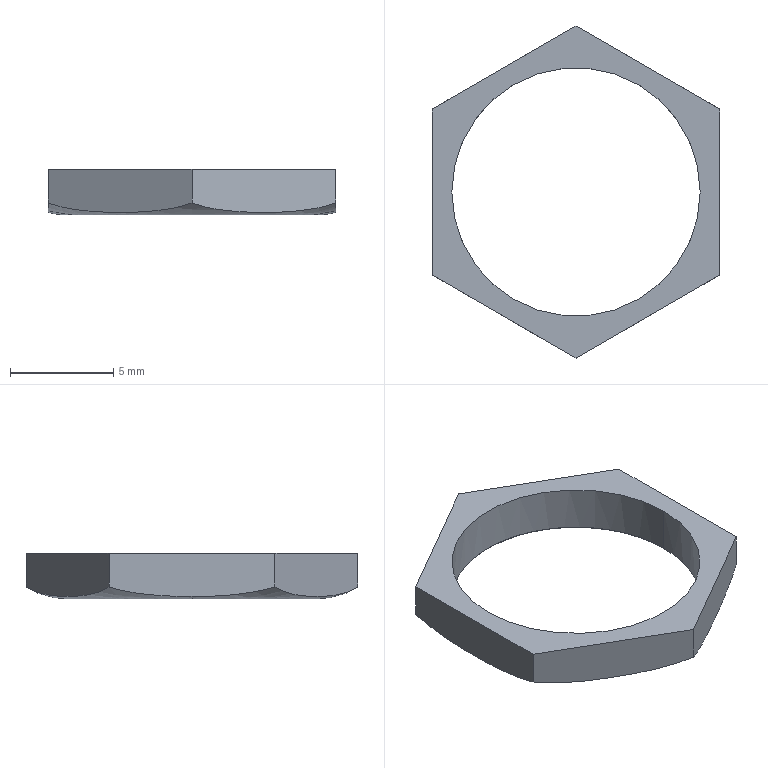Part | SolidWorks | 1 solid | 12 faces | box 13.895 x 16.044 x 2.21 mm | volume 114.581 mm3 | plane 8 | spline 2 | cylinder 2 | commonest cylinder face diameters 12 x2
STEP:
#1=CARTESIAN_POINT('',(6.,-0.00001674,-2.83));
#2=VERTEX_POINT('',#1);
#3=CARTESIAN_POINT('',(-6.,-0.00001674,-2.83));
#4=VERTEX_POINT('',#3);
#5=CARTESIAN_POINT('',(0.,-0.00001674,-2.83));
#6=DIRECTION('',(0.,0.,1.));
#7=DIRECTION('',(1.,0.,0.));
#8=AXIS2_PLACEMENT_3D('',#5,#6,#7);
#9=CIRCLE('',#8,6.);
#10=EDGE_CURVE('',#2,#4,#9,.T.);
#11=ORIENTED_EDGE('',*,*,#10,.T.);
#12=CARTESIAN_POINT('',(0.,-0.00001674,-2.83));
#13=DIRECTION('',(0.,0.,1.));
#14=DIRECTION('',(1.,0.,0.));
#15=AXIS2_PLACEMENT_3D('',#12,#13,#14);
#16=CIRCLE('',#15,6.);
#17=EDGE_CURVE('',#4,#2,#16,.T.);
#18=ORIENTED_EDGE('',*,*,#17,.T.);
#19=EDGE_LOOP('',(#11,#18));
#20=FACE_BOUND('',#19,.T.);
#21=CARTESIAN_POINT('',(-6.017,-0.00001674,-2.83));
#22=VERTEX_POINT('',#21);
#23=CARTESIAN_POINT('',(6.017,-0.00001674,-2.83));
#24=VERTEX_POINT('',#23);
#25=CARTESIAN_POINT('',(-6.017,-0.00001674,-2.83));
#26=CARTESIAN_POINT('',(-6.017,-12.033,-2.83));
#27=CARTESIAN_POINT('',(6.017,-12.033,-2.83));
#28=CARTESIAN_POINT('',(6.017,-0.00001674,-2.83));
#29=(BOUNDED_CURVE()B_SPLINE_CURVE(3,(#25,#26,#27,#28),.UNSPECIFIED.,.F.,.T.)B_SPLINE_CURVE_WITH_KNOTS((4,4),(0.,1.),.UNSPECIFIED.)CURVE()GEOMETRIC_REPRESENTATION_ITEM()RATIONAL_B_SPLINE_CURVE((1.,0.3333,0.3333,1.))REPRESENTATION_ITEM(''));
#30=EDGE_CURVE('',#22,#24,#29,.T.);
#31=ORIENTED_EDGE('',*,*,#30,.F.);
#32=CARTESIAN_POINT('',(6.017,-0.00001674,-2.83));
#33=CARTESIAN_POINT('',(6.017,12.033,-2.83));
#34=CARTESIAN_POINT('',(-6.017,12.033,-2.83));
#35=CARTESIAN_POINT('',(-6.017,-0.00001674,-2.83));
#36=(BOUNDED_CURVE()B_SPLINE_CURVE(3,(#32,#33,#34,#35),.UNSPECIFIED.,.F.,.T.)B_SPLINE_CURVE_WITH_KNOTS((4,4),(0.,1.),.UNSPECIFIED.)CURVE()GEOMETRIC_REPRESENTATION_ITEM()RATIONAL_B_SPLINE_CURVE((1.,0.3333,0.3333,1.))REPRESENTATION_ITEM(''));
#37=EDGE_CURVE('',#24,#22,#36,.T.);
#38=ORIENTED_EDGE('',*,*,#37,.F.);
#39=EDGE_LOOP('',(#31,#38));
#40=FACE_OUTER_BOUND('',#39,.T.);
#41=CARTESIAN_POINT('',(0.,6.016,-2.83));
#42=DIRECTION('',(0.,0.,1.));
#43=DIRECTION('',(1.,0.,0.));
#44=AXIS2_PLACEMENT_3D('',#41,#42,#43);
#45=PLANE('',#44);
#46=ADVANCED_FACE('',(#20,#40),#45,.F.);
#47=CARTESIAN_POINT('',(-6.947,-0.00001674,-2.715));
#48=VERTEX_POINT('',#47);
#49=CARTESIAN_POINT('',(-6.017,-0.00001674,0.9919));
#50=DIRECTION('',(0.,-1.,0.));
#51=DIRECTION('',(-1.,0.,0.));
#52=AXIS2_PLACEMENT_3D('',#49,#50,#51);
#53=CIRCLE('',#52,3.822);
#54=EDGE_CURVE('',#48,#22,#53,.T.);
#55=ORIENTED_EDGE('',*,*,#54,.F.);
#56=CARTESIAN_POINT('',(-6.947,4.011,-2.262));
#57=VERTEX_POINT('',#56);
#58=CARTESIAN_POINT('',(-6.947,4.011,-2.262));
#59=CARTESIAN_POINT('',(-6.947,3.728,-2.349));
#60=CARTESIAN_POINT('',(-6.947,3.267,-2.46));
#61=CARTESIAN_POINT('',(-6.947,2.666,-2.557));
#62=CARTESIAN_POINT('',(-6.947,2.349,-2.597));
#63=CARTESIAN_POINT('',(-6.947,2.187,-2.614));
#64=CARTESIAN_POINT('',(-6.947,2.104,-2.623));
#65=CARTESIAN_POINT('',(-6.947,2.063,-2.627));
#66=CARTESIAN_POINT('',(-6.947,2.045,-2.628));
#67=CARTESIAN_POINT('',(-6.947,2.033,-2.63));
#68=CARTESIAN_POINT('',(-6.947,2.026,-2.63));
#69=CARTESIAN_POINT('',(-6.947,1.422,-2.687));
#70=CARTESIAN_POINT('',(-6.947,0.7486,-2.715));
#71=CARTESIAN_POINT('',(-6.947,-0.00001674,-2.715));
#72=B_SPLINE_CURVE_WITH_KNOTS('',3,(#58,#59,#60,#61,#62,#63,#64,#65,#66,#67,#68,#69,#70,#71),.UNSPECIFIED.,.F.,.F.,(4,1,1,1,1,1,1,2,2,4),(0.,0.25,0.375,0.4375,0.4688,0.4844,0.4922,0.4961,0.5,1.),.UNSPECIFIED.);
#73=EDGE_CURVE('',#57,#48,#72,.T.);
#74=ORIENTED_EDGE('',*,*,#73,.F.);
#75=CARTESIAN_POINT('',(0.,8.022,-2.262));
#76=VERTEX_POINT('',#75);
#77=CARTESIAN_POINT('',(0.,8.022,-2.262));
#78=CARTESIAN_POINT('',(-0.245,7.881,-2.349));
#79=CARTESIAN_POINT('',(-0.6442,7.65,-2.461));
#80=CARTESIAN_POINT('',(-1.165,7.349,-2.557));
#81=CARTESIAN_POINT('',(-1.439,7.191,-2.597));
#82=CARTESIAN_POINT('',(-1.58,7.11,-2.614));
#83=CARTESIAN_POINT('',(-1.651,7.069,-2.623));
#84=CARTESIAN_POINT('',(-1.687,7.048,-2.627));
#85=CARTESIAN_POINT('',(-1.702,7.039,-2.628));
#86=CARTESIAN_POINT('',(-1.713,7.033,-2.63));
#87=CARTESIAN_POINT('',(-1.719,7.03,-2.63));
#88=CARTESIAN_POINT('',(-2.242,6.728,-2.687));
#89=CARTESIAN_POINT('',(-2.826,6.391,-2.715));
#90=CARTESIAN_POINT('',(-3.797,5.83,-2.715));
#91=CARTESIAN_POINT('',(-4.259,5.563,-2.705));
#92=CARTESIAN_POINT('',(-4.756,5.276,-2.674));
#93=CARTESIAN_POINT('',(-4.994,5.139,-2.654));
#94=CARTESIAN_POINT('',(-5.11,5.072,-2.643));
#95=CARTESIAN_POINT('',(-5.167,5.039,-2.637));
#96=CARTESIAN_POINT('',(-5.196,5.022,-2.634));
#97=CARTESIAN_POINT('',(-5.208,5.015,-2.632));
#98=CARTESIAN_POINT('',(-5.216,5.01,-2.632));
#99=CARTESIAN_POINT('',(-5.219,5.009,-2.631));
#100=CARTESIAN_POINT('',(-5.883,4.626,-2.559));
#101=CARTESIAN_POINT('',(-6.457,4.294,-2.436));
#102=CARTESIAN_POINT('',(-6.947,4.011,-2.262));
#103=B_SPLINE_CURVE_WITH_KNOTS('',3,(#77,#78,#79,#80,#81,#82,#83,#84,#85,#86,#87,#88,#89,#90,#91,#92,#93,#94,#95,#96,#97,#98,#99,#100,#101,#102),.UNSPECIFIED.,.F.,.F.,(4,1,1,1,1,1,1,2,2,2,1,1,1,1,1,1,2,2,4),(0.,0.125,0.1875,0.2187,0.2344,0.2422,0.2461,0.248,0.25,0.5,0.625,0.6875,0.7187,0.7344,0.7422,0.7461,0.748,0.75,1.),.UNSPECIFIED.);
#104=EDGE_CURVE('',#76,#57,#103,.T.);
#105=ORIENTED_EDGE('',*,*,#104,.F.);
#106=CARTESIAN_POINT('',(6.947,4.011,-2.262));
#107=VERTEX_POINT('',#106);
#108=CARTESIAN_POINT('',(6.947,4.011,-2.262));
#109=CARTESIAN_POINT('',(6.702,4.152,-2.349));
#110=CARTESIAN_POINT('',(6.303,4.383,-2.461));
#111=CARTESIAN_POINT('',(5.782,4.684,-2.557));
#112=CARTESIAN_POINT('',(5.508,4.842,-2.597));
#113=CARTESIAN_POINT('',(5.367,4.923,-2.614));
#114=CARTESIAN_POINT('',(5.296,4.964,-2.623));
#115=CARTESIAN_POINT('',(5.26,4.985,-2.627));
#116=CARTESIAN_POINT('',(5.245,4.994,-2.628));
#117=CARTESIAN_POINT('',(5.235,5.,-2.63));
#118=CARTESIAN_POINT('',(5.228,5.003,-2.63));
#119=CARTESIAN_POINT('',(4.706,5.305,-2.687));
#120=CARTESIAN_POINT('',(4.122,5.642,-2.715));
#121=CARTESIAN_POINT('',(3.15,6.203,-2.715));
#122=CARTESIAN_POINT('',(2.688,6.47,-2.705));
#123=CARTESIAN_POINT('',(2.191,6.757,-2.674));
#124=CARTESIAN_POINT('',(1.954,6.894,-2.654));
#125=CARTESIAN_POINT('',(1.837,6.961,-2.643));
#126=CARTESIAN_POINT('',(1.78,6.994,-2.637));
#127=CARTESIAN_POINT('',(1.751,7.011,-2.634));
#128=CARTESIAN_POINT('',(1.739,7.018,-2.632));
#129=CARTESIAN_POINT('',(1.731,7.023,-2.632));
#130=CARTESIAN_POINT('',(1.728,7.024,-2.631));
#131=CARTESIAN_POINT('',(1.065,7.407,-2.559));
#132=CARTESIAN_POINT('',(0.4902,7.739,-2.436));
#133=CARTESIAN_POINT('',(0.,8.022,-2.262));
#134=B_SPLINE_CURVE_WITH_KNOTS('',3,(#108,#109,#110,#111,#112,#113,#114,#115,#116,#117,#118,#119,#120,#121,#122,#123,#124,#125,#126,#127,#128,#129,#130,#131,#132,#133),.UNSPECIFIED.,.F.,.F.,(4,1,1,1,1,1,1,2,2,2,1,1,1,1,1,1,2,2,4),(0.,0.125,0.1875,0.2188,0.2344,0.2422,0.2461,0.248,0.25,0.5,0.625,0.6875,0.7187,0.7344,0.7422,0.7461,0.748,0.75,1.),.UNSPECIFIED.);
#135=EDGE_CURVE('',#107,#76,#134,.T.);
#136=ORIENTED_EDGE('',*,*,#135,.F.);
#137=CARTESIAN_POINT('',(6.947,-0.00001674,-2.715));
#138=VERTEX_POINT('',#137);
#139=CARTESIAN_POINT('',(6.947,-0.00001674,-2.715));
#140=CARTESIAN_POINT('',(6.947,0.3741,-2.715));
#141=CARTESIAN_POINT('',(6.947,0.9074,-2.705));
#142=CARTESIAN_POINT('',(6.947,1.481,-2.674));
#143=CARTESIAN_POINT('',(6.947,1.755,-2.654));
#144=CARTESIAN_POINT('',(6.947,1.889,-2.643));
#145=CARTESIAN_POINT('',(6.947,1.956,-2.637));
#146=CARTESIAN_POINT('',(6.947,1.989,-2.634));
#147=CARTESIAN_POINT('',(6.947,2.003,-2.632));
#148=CARTESIAN_POINT('',(6.947,2.012,-2.632));
#149=CARTESIAN_POINT('',(6.947,2.016,-2.631));
#150=CARTESIAN_POINT('',(6.947,2.782,-2.559));
#151=CARTESIAN_POINT('',(6.947,3.445,-2.436));
#152=CARTESIAN_POINT('',(6.947,4.011,-2.262));
#153=B_SPLINE_CURVE_WITH_KNOTS('',3,(#139,#140,#141,#142,#143,#144,#145,#146,#147,#148,#149,#150,#151,#152),.UNSPECIFIED.,.F.,.F.,(4,1,1,1,1,1,1,2,2,4),(0.,0.25,0.375,0.4375,0.4688,0.4844,0.4922,0.4961,0.5,1.),.UNSPECIFIED.);
#154=EDGE_CURVE('',#138,#107,#153,.T.);
#155=ORIENTED_EDGE('',*,*,#154,.F.);
#156=CARTESIAN_POINT('',(6.017,-0.00001674,0.9919));
#157=DIRECTION('',(0.,1.,0.));
#158=DIRECTION('',(1.,0.,0.));
#159=AXIS2_PLACEMENT_3D('',#156,#157,#158);
#160=CIRCLE('',#159,3.822);
#161=EDGE_CURVE('',#138,#24,#160,.T.);
#162=ORIENTED_EDGE('',*,*,#161,.T.);
#163=ORIENTED_EDGE('',*,*,#37,.T.);
#164=EDGE_LOOP('',(#55,#74,#105,#136,#155,#162,#163));
#165=FACE_OUTER_BOUND('',#164,.T.);
#166=CARTESIAN_POINT('',(8.033,-0.00001674,-2.255));
#167=CARTESIAN_POINT('',(8.033,16.066,-2.255));
#168=CARTESIAN_POINT('',(-8.033,16.066,-2.255));
#169=CARTESIAN_POINT('',(-8.033,-0.00001674,-2.255));
#170=CARTESIAN_POINT('',(7.423,-0.00001674,-2.633));
#171=CARTESIAN_POINT('',(7.423,14.847,-2.633));
#172=CARTESIAN_POINT('',(-7.423,14.847,-2.633));
#173=CARTESIAN_POINT('',(-7.423,-0.00001674,-2.633));
#174=CARTESIAN_POINT('',(6.734,-0.00001674,-2.83));
#175=CARTESIAN_POINT('',(6.734,13.467,-2.83));
#176=CARTESIAN_POINT('',(-6.734,13.467,-2.83));
#177=CARTESIAN_POINT('',(-6.734,-0.00001674,-2.83));
#178=CARTESIAN_POINT('',(6.017,-0.00001674,-2.83));
#179=CARTESIAN_POINT('',(6.017,12.033,-2.83));
#180=CARTESIAN_POINT('',(-6.017,12.033,-2.83));
#181=CARTESIAN_POINT('',(-6.017,-0.00001674,-2.83));
#182=(BOUNDED_SURFACE()B_SPLINE_SURFACE(3,3,((#166,#167,#168,#169),(#170,#171,#172,#173),(#174,#175,#176,#177),(#178,#179,#180,#181)),.UNSPECIFIED.,.F.,.F.,.F.)B_SPLINE_SURFACE_WITH_KNOTS((4,4),(4,4),(0.,1.),(0.,1.),.UNSPECIFIED.)GEOMETRIC_REPRESENTATION_ITEM()RATIONAL_B_SPLINE_SURFACE(((1.,0.3333,0.3333,1.),(0.9744,0.3248,0.3248,0.9744),(0.9744,0.3248,0.3248,0.9744),(1.,0.3333,0.3333,1.)))REPRESENTATION_ITEM('')SURFACE());
#183=ADVANCED_FACE('',(#165),#182,.T.);
#184=CARTESIAN_POINT('',(-6.,-0.00001674,-0.6197));
#185=VERTEX_POINT('',#184);
#186=CARTESIAN_POINT('',(-6.,-0.00001674,-0.6197));
#187=DIRECTION('',(0.,0.,1.));
#188=VECTOR('',#187,1000.);
#189=LINE('',#186,#188);
#190=EDGE_CURVE('',#4,#185,#189,.T.);
#191=ORIENTED_EDGE('',*,*,#190,.F.);
#192=ORIENTED_EDGE('',*,*,#10,.F.);
#193=CARTESIAN_POINT('',(6.,-0.00001674,-0.6197));
#194=VERTEX_POINT('',#193);
#195=CARTESIAN_POINT('',(6.,-0.00001674,-0.6197));
#196=DIRECTION('',(0.,0.,1.));
#197=VECTOR('',#196,1000.);
#198=LINE('',#195,#197);
#199=EDGE_CURVE('',#2,#194,#198,.T.);
#200=ORIENTED_EDGE('',*,*,#199,.T.);
#201=CARTESIAN_POINT('',(0.,-0.00001674,-0.6197));
#202=DIRECTION('',(0.,0.,1.));
#203=DIRECTION('',(1.,0.,0.));
#204=AXIS2_PLACEMENT_3D('',#201,#202,#203);
#205=CIRCLE('',#204,6.);
#206=EDGE_CURVE('',#194,#185,#205,.T.);
#207=ORIENTED_EDGE('',*,*,#206,.T.);
#208=EDGE_LOOP('',(#191,#192,#200,#207));
#209=FACE_OUTER_BOUND('',#208,.T.);
#210=CARTESIAN_POINT('',(0.,-0.00001674,-0.6197));
#211=DIRECTION('',(0.,0.,1.));
#212=DIRECTION('',(1.,0.,0.));
#213=AXIS2_PLACEMENT_3D('',#210,#211,#212);
#214=CYLINDRICAL_SURFACE('',#213,6.);
#215=ADVANCED_FACE('',(#209),#214,.F.);
#216=CARTESIAN_POINT('',(6.947,4.011,-0.6197));
#217=VERTEX_POINT('',#216);
#218=CARTESIAN_POINT('',(6.947,-4.011,-0.6197));
#219=VERTEX_POINT('',#218);
#220=CARTESIAN_POINT('',(6.947,6.,-0.6197));
#221=DIRECTION('',(0.,-1.,0.));
#222=VECTOR('',#221,1000.);
#223=LINE('',#220,#222);
#224=EDGE_CURVE('',#217,#219,#223,.T.);
#225=ORIENTED_EDGE('',*,*,#224,.T.);
#226=CARTESIAN_POINT('',(6.947,-4.011,-2.262));
#227=VERTEX_POINT('',#226);
#228=CARTESIAN_POINT('',(6.947,-4.011,-2.83));
#229=DIRECTION('',(0.,0.,1.));
#230=VECTOR('',#229,1000.);
#231=LINE('',#228,#230);
#232=EDGE_CURVE('',#227,#219,#231,.T.);
#233=ORIENTED_EDGE('',*,*,#232,.F.);
#234=CARTESIAN_POINT('',(6.947,-4.011,-2.262));
#235=CARTESIAN_POINT('',(6.947,-3.728,-2.349));
#236=CARTESIAN_POINT('',(6.947,-3.267,-2.46));
#237=CARTESIAN_POINT('',(6.947,-2.666,-2.557));
#238=CARTESIAN_POINT('',(6.947,-2.349,-2.597));
#239=CARTESIAN_POINT('',(6.947,-2.187,-2.614));
#240=CARTESIAN_POINT('',(6.947,-2.104,-2.623));
#241=CARTESIAN_POINT('',(6.947,-2.063,-2.627));
#242=CARTESIAN_POINT('',(6.947,-2.045,-2.628));
#243=CARTESIAN_POINT('',(6.947,-2.033,-2.63));
#244=CARTESIAN_POINT('',(6.947,-2.026,-2.63));
#245=CARTESIAN_POINT('',(6.947,-1.423,-2.687));
#246=CARTESIAN_POINT('',(6.947,-0.7487,-2.715));
#247=CARTESIAN_POINT('',(6.947,-0.00001674,-2.715));
#248=B_SPLINE_CURVE_WITH_KNOTS('',3,(#234,#235,#236,#237,#238,#239,#240,#241,#242,#243,#244,#245,#246,#247),.UNSPECIFIED.,.F.,.F.,(4,1,1,1,1,1,1,2,2,4),(0.,0.25,0.375,0.4375,0.4687,0.4844,0.4922,0.4961,0.5,1.),.UNSPECIFIED.);
#249=EDGE_CURVE('',#227,#138,#248,.T.);
#250=ORIENTED_EDGE('',*,*,#249,.T.);
#251=ORIENTED_EDGE('',*,*,#154,.T.);
#252=CARTESIAN_POINT('',(6.947,4.011,-2.83));
#253=DIRECTION('',(0.,0.,-1.));
#254=VECTOR('',#253,1000.);
#255=LINE('',#252,#254);
#256=EDGE_CURVE('',#217,#107,#255,.T.);
#257=ORIENTED_EDGE('',*,*,#256,.F.);
#258=EDGE_LOOP('',(#225,#233,#250,#251,#257));
#259=FACE_OUTER_BOUND('',#258,.T.);
#260=CARTESIAN_POINT('',(6.947,-4.011,-2.83));
#261=DIRECTION('',(1.,0.,0.));
#262=DIRECTION('',(0.,1.,0.));
#263=AXIS2_PLACEMENT_3D('',#260,#261,#262);
#264=PLANE('',#263);
#265=ADVANCED_FACE('',(#259),#264,.T.);
#266=CARTESIAN_POINT('',(0.,-8.022,-0.6197));
#267=VERTEX_POINT('',#266);
#268=CARTESIAN_POINT('',(6.947,-4.011,-0.6197));
#269=DIRECTION('',(-0.866,-0.5,0.));
#270=VECTOR('',#269,1000.);
#271=LINE('',#268,#270);
#272=EDGE_CURVE('',#219,#267,#271,.T.);
#273=ORIENTED_EDGE('',*,*,#272,.T.);
#274=CARTESIAN_POINT('',(0.,-8.022,-2.262));
#275=VERTEX_POINT('',#274);
#276=CARTESIAN_POINT('',(0.,-8.022,-2.83));
#277=DIRECTION('',(0.,0.,1.));
#278=VECTOR('',#277,1000.);
#279=LINE('',#276,#278);
#280=EDGE_CURVE('',#275,#267,#279,.T.);
#281=ORIENTED_EDGE('',*,*,#280,.F.);
#282=CARTESIAN_POINT('',(0.,-8.022,-2.262));
#283=CARTESIAN_POINT('',(0.245,-7.881,-2.349));
#284=CARTESIAN_POINT('',(0.6442,-7.65,-2.461));
#285=CARTESIAN_POINT('',(1.165,-7.349,-2.557));
#286=CARTESIAN_POINT('',(1.439,-7.191,-2.597));
#287=CARTESIAN_POINT('',(1.58,-7.11,-2.614));
#288=CARTESIAN_POINT('',(1.651,-7.069,-2.623));
#289=CARTESIAN_POINT('',(1.687,-7.048,-2.627));
#290=CARTESIAN_POINT('',(1.702,-7.039,-2.628));
#291=CARTESIAN_POINT('',(1.713,-7.033,-2.63));
#292=CARTESIAN_POINT('',(1.719,-7.03,-2.63));
#293=CARTESIAN_POINT('',(2.242,-6.728,-2.687));
#294=CARTESIAN_POINT('',(2.826,-6.391,-2.715));
#295=CARTESIAN_POINT('',(3.797,-5.83,-2.715));
#296=CARTESIAN_POINT('',(4.259,-5.563,-2.705));
#297=CARTESIAN_POINT('',(4.756,-5.276,-2.674));
#298=CARTESIAN_POINT('',(4.994,-5.139,-2.654));
#299=CARTESIAN_POINT('',(5.11,-5.072,-2.643));
#300=CARTESIAN_POINT('',(5.167,-5.039,-2.637));
#301=CARTESIAN_POINT('',(5.196,-5.022,-2.634));
#302=CARTESIAN_POINT('',(5.208,-5.015,-2.632));
#303=CARTESIAN_POINT('',(5.216,-5.01,-2.632));
#304=CARTESIAN_POINT('',(5.219,-5.009,-2.631));
#305=CARTESIAN_POINT('',(5.883,-4.626,-2.559));
#306=CARTESIAN_POINT('',(6.457,-4.294,-2.436));
#307=CARTESIAN_POINT('',(6.947,-4.011,-2.262));
#308=B_SPLINE_CURVE_WITH_KNOTS('',3,(#282,#283,#284,#285,#286,#287,#288,#289,#290,#291,#292,#293,#294,#295,#296,#297,#298,#299,#300,#301,#302,#303,#304,#305,#306,#307),.UNSPECIFIED.,.F.,.F.,(4,1,1,1,1,1,1,2,2,2,1,1,1,1,1,1,2,2,4),(0.,0.125,0.1875,0.2188,0.2344,0.2422,0.2461,0.248,0.25,0.5,0.625,0.6875,0.7187,0.7344,0.7422,0.7461,0.748,0.75,1.),.UNSPECIFIED.);
#309=EDGE_CURVE('',#275,#227,#308,.T.);
#310=ORIENTED_EDGE('',*,*,#309,.T.);
#311=ORIENTED_EDGE('',*,*,#232,.T.);
#312=EDGE_LOOP('',(#273,#281,#310,#311));
#313=FACE_OUTER_BOUND('',#312,.T.);
#314=CARTESIAN_POINT('',(0.,-8.022,-2.83));
#315=DIRECTION('',(0.5,-0.866,0.));
#316=DIRECTION('',(0.,0.,-1.));
#317=AXIS2_PLACEMENT_3D('',#314,#315,#316);
#318=PLANE('',#317);
#319=ADVANCED_FACE('',(#313),#318,.T.);
#320=CARTESIAN_POINT('',(-6.947,-4.011,-0.6197));
#321=VERTEX_POINT('',#320);
#322=CARTESIAN_POINT('',(0.,-8.022,-0.6197));
#323=DIRECTION('',(-0.866,0.5,0.));
#324=VECTOR('',#323,1000.);
#325=LINE('',#322,#324);
#326=EDGE_CURVE('',#267,#321,#325,.T.);
#327=ORIENTED_EDGE('',*,*,#326,.T.);
#328=CARTESIAN_POINT('',(-6.947,-4.011,-2.262));
#329=VERTEX_POINT('',#328);
#330=CARTESIAN_POINT('',(-6.947,-4.011,-2.83));
#331=DIRECTION('',(0.,0.,1.));
#332=VECTOR('',#331,1000.);
#333=LINE('',#330,#332);
#334=EDGE_CURVE('',#329,#321,#333,.T.);
#335=ORIENTED_EDGE('',*,*,#334,.F.);
#336=CARTESIAN_POINT('',(-6.947,-4.011,-2.262));
#337=CARTESIAN_POINT('',(-6.702,-4.152,-2.349));
#338=CARTESIAN_POINT('',(-6.303,-4.383,-2.461));
#339=CARTESIAN_POINT('',(-5.782,-4.684,-2.557));
#340=CARTESIAN_POINT('',(-5.508,-4.842,-2.597));
#341=CARTESIAN_POINT('',(-5.367,-4.923,-2.614));
#342=CARTESIAN_POINT('',(-5.296,-4.964,-2.623));
#343=CARTESIAN_POINT('',(-5.26,-4.985,-2.627));
#344=CARTESIAN_POINT('',(-5.245,-4.994,-2.628));
#345=CARTESIAN_POINT('',(-5.235,-5.,-2.63));
#346=CARTESIAN_POINT('',(-5.228,-5.003,-2.63));
#347=CARTESIAN_POINT('',(-4.706,-5.305,-2.687));
#348=CARTESIAN_POINT('',(-4.122,-5.642,-2.715));
#349=CARTESIAN_POINT('',(-3.15,-6.204,-2.715));
#350=CARTESIAN_POINT('',(-2.688,-6.47,-2.705));
#351=CARTESIAN_POINT('',(-2.191,-6.757,-2.674));
#352=CARTESIAN_POINT('',(-1.954,-6.894,-2.654));
#353=CARTESIAN_POINT('',(-1.837,-6.961,-2.643));
#354=CARTESIAN_POINT('',(-1.78,-6.994,-2.637));
#355=CARTESIAN_POINT('',(-1.751,-7.011,-2.634));
#356=CARTESIAN_POINT('',(-1.739,-7.018,-2.632));
#357=CARTESIAN_POINT('',(-1.731,-7.023,-2.632));
#358=CARTESIAN_POINT('',(-1.728,-7.024,-2.631));
#359=CARTESIAN_POINT('',(-1.065,-7.407,-2.559));
#360=CARTESIAN_POINT('',(-0.4902,-7.739,-2.436));
#361=CARTESIAN_POINT('',(0.,-8.022,-2.262));
#362=B_SPLINE_CURVE_WITH_KNOTS('',3,(#336,#337,#338,#339,#340,#341,#342,#343,#344,#345,#346,#347,#348,#349,#350,#351,#352,#353,#354,#355,#356,#357,#358,#359,#360,#361),.UNSPECIFIED.,.F.,.F.,(4,1,1,1,1,1,1,2,2,2,1,1,1,1,1,1,2,2,4),(0.,0.125,0.1875,0.2187,0.2344,0.2422,0.2461,0.248,0.25,0.5,0.625,0.6875,0.7188,0.7344,0.7422,0.7461,0.748,0.75,1.),.UNSPECIFIED.);
#363=EDGE_CURVE('',#329,#275,#362,.T.);
#364=ORIENTED_EDGE('',*,*,#363,.T.);
#365=ORIENTED_EDGE('',*,*,#280,.T.);
#366=EDGE_LOOP('',(#327,#335,#364,#365));
#367=FACE_OUTER_BOUND('',#366,.T.);
#368=CARTESIAN_POINT('',(-6.947,-4.011,-2.83));
#369=DIRECTION('',(-0.5,-0.866,0.));
#370=DIRECTION('',(-0.866,0.5,0.));
#371=AXIS2_PLACEMENT_3D('',#368,#369,#370);
#372=PLANE('',#371);
#373=ADVANCED_FACE('',(#367),#372,.T.);
#374=CARTESIAN_POINT('',(-6.947,4.011,-0.6197));
#375=VERTEX_POINT('',#374);
#376=CARTESIAN_POINT('',(-6.947,6.,-0.6197));
#377=DIRECTION('',(0.,1.,0.));
#378=VECTOR('',#377,1000.);
#379=LINE('',#376,#378);
#380=EDGE_CURVE('',#321,#375,#379,.T.);
#381=ORIENTED_EDGE('',*,*,#380,.T.);
#382=CARTESIAN_POINT('',(-6.947,4.011,-2.83));
#383=DIRECTION('',(0.,0.,1.));
#384=VECTOR('',#383,1000.);
#385=LINE('',#382,#384);
#386=EDGE_CURVE('',#57,#375,#385,.T.);
#387=ORIENTED_EDGE('',*,*,#386,.F.);
#388=ORIENTED_EDGE('',*,*,#73,.T.);
#389=CARTESIAN_POINT('',(-6.947,-0.00001674,-2.715));
#390=CARTESIAN_POINT('',(-6.947,-0.3741,-2.715));
#391=CARTESIAN_POINT('',(-6.947,-0.9074,-2.705));
#392=CARTESIAN_POINT('',(-6.947,-1.481,-2.674));
#393=CARTESIAN_POINT('',(-6.947,-1.755,-2.654));
#394=CARTESIAN_POINT('',(-6.947,-1.889,-2.643));
#395=CARTESIAN_POINT('',(-6.947,-1.956,-2.637));
#396=CARTESIAN_POINT('',(-6.947,-1.989,-2.634));
#397=CARTESIAN_POINT('',(-6.947,-2.003,-2.632));
#398=CARTESIAN_POINT('',(-6.947,-2.012,-2.632));
#399=CARTESIAN_POINT('',(-6.947,-2.016,-2.631));
#400=CARTESIAN_POINT('',(-6.947,-2.782,-2.559));
#401=CARTESIAN_POINT('',(-6.947,-3.445,-2.436));
#402=CARTESIAN_POINT('',(-6.947,-4.011,-2.262));
#403=B_SPLINE_CURVE_WITH_KNOTS('',3,(#389,#390,#391,#392,#393,#394,#395,#396,#397,#398,#399,#400,#401,#402),.UNSPECIFIED.,.F.,.F.,(4,1,1,1,1,1,1,2,2,4),(0.,0.25,0.375,0.4375,0.4687,0.4844,0.4922,0.4961,0.5,1.),.UNSPECIFIED.);
#404=EDGE_CURVE('',#48,#329,#403,.T.);
#405=ORIENTED_EDGE('',*,*,#404,.T.);
#406=ORIENTED_EDGE('',*,*,#334,.T.);
#407=EDGE_LOOP('',(#381,#387,#388,#405,#406));
#408=FACE_OUTER_BOUND('',#407,.T.);
#409=CARTESIAN_POINT('',(-6.947,4.011,-2.83));
#410=DIRECTION('',(-1.,0.,0.));
#411=DIRECTION('',(0.,1.,0.));
#412=AXIS2_PLACEMENT_3D('',#409,#410,#411);
#413=PLANE('',#412);
#414=ADVANCED_FACE('',(#408),#413,.T.);
#415=CARTESIAN_POINT('',(0.,8.022,-0.6197));
#416=VERTEX_POINT('',#415);
#417=CARTESIAN_POINT('',(-6.947,4.011,-0.6197));
#418=DIRECTION('',(0.866,0.5,0.));
#419=VECTOR('',#418,1000.);
#420=LINE('',#417,#419);
#421=EDGE_CURVE('',#375,#416,#420,.T.);
#422=ORIENTED_EDGE('',*,*,#421,.T.);
#423=CARTESIAN_POINT('',(0.,8.022,-2.83));
#424=DIRECTION('',(0.,0.,1.));
#425=VECTOR('',#424,1000.);
#426=LINE('',#423,#425);
#427=EDGE_CURVE('',#76,#416,#426,.T.);
#428=ORIENTED_EDGE('',*,*,#427,.F.);
#429=ORIENTED_EDGE('',*,*,#104,.T.);
#430=ORIENTED_EDGE('',*,*,#386,.T.);
#431=EDGE_LOOP('',(#422,#428,#429,#430));
#432=FACE_OUTER_BOUND('',#431,.T.);
#433=CARTESIAN_POINT('',(0.,8.022,-2.83));
#434=DIRECTION('',(-0.5,0.866,0.));
#435=DIRECTION('',(0.,0.,1.));
#436=AXIS2_PLACEMENT_3D('',#433,#434,#435);
#437=PLANE('',#436);
#438=ADVANCED_FACE('',(#432),#437,.T.);
#439=CARTESIAN_POINT('',(0.,8.022,-0.6197));
#440=DIRECTION('',(0.866,-0.5,0.));
#441=VECTOR('',#440,1000.);
#442=LINE('',#439,#441);
#443=EDGE_CURVE('',#416,#217,#442,.T.);
#444=ORIENTED_EDGE('',*,*,#443,.T.);
#445=ORIENTED_EDGE('',*,*,#256,.T.);
#446=ORIENTED_EDGE('',*,*,#135,.T.);
#447=ORIENTED_EDGE('',*,*,#427,.T.);
#448=EDGE_LOOP('',(#444,#445,#446,#447));
#449=FACE_OUTER_BOUND('',#448,.T.);
#450=CARTESIAN_POINT('',(6.947,4.011,-2.83));
#451=DIRECTION('',(0.5,0.866,0.));
#452=DIRECTION('',(0.,0.,-1.));
#453=AXIS2_PLACEMENT_3D('',#450,#451,#452);
#454=PLANE('',#453);
#455=ADVANCED_FACE('',(#449),#454,.T.);
#456=ORIENTED_EDGE('',*,*,#206,.F.);
#457=CARTESIAN_POINT('',(0.,-0.00001674,-0.6197));
#458=DIRECTION('',(0.,0.,1.));
#459=DIRECTION('',(1.,0.,0.));
#460=AXIS2_PLACEMENT_3D('',#457,#458,#459);
#461=CIRCLE('',#460,6.);
#462=EDGE_CURVE('',#185,#194,#461,.T.);
#463=ORIENTED_EDGE('',*,*,#462,.F.);
#464=EDGE_LOOP('',(#456,#463));
#465=FACE_BOUND('',#464,.T.);
#466=ORIENTED_EDGE('',*,*,#421,.F.);
#467=ORIENTED_EDGE('',*,*,#380,.F.);
#468=ORIENTED_EDGE('',*,*,#326,.F.);
#469=ORIENTED_EDGE('',*,*,#272,.F.);
#470=ORIENTED_EDGE('',*,*,#224,.F.);
#471=ORIENTED_EDGE('',*,*,#443,.F.);
#472=EDGE_LOOP('',(#466,#467,#468,#469,#470,#471));
#473=FACE_OUTER_BOUND('',#472,.T.);
#474=CARTESIAN_POINT('',(0.,6.,-0.6197));
#475=DIRECTION('',(0.,0.,-1.));
#476=DIRECTION('',(0.,-1.,0.));
#477=AXIS2_PLACEMENT_3D('',#474,#475,#476);
#478=PLANE('',#477);
#479=ADVANCED_FACE('',(#465,#473),#478,.F.);
#480=ORIENTED_EDGE('',*,*,#17,.F.);
#481=ORIENTED_EDGE('',*,*,#190,.T.);
#482=ORIENTED_EDGE('',*,*,#462,.T.);
#483=ORIENTED_EDGE('',*,*,#199,.F.);
#484=EDGE_LOOP('',(#480,#481,#482,#483));
#485=FACE_OUTER_BOUND('',#484,.T.);
#486=CARTESIAN_POINT('',(0.,-0.00001674,-0.6197));
#487=DIRECTION('',(0.,0.,1.));
#488=DIRECTION('',(1.,0.,0.));
#489=AXIS2_PLACEMENT_3D('',#486,#487,#488);
#490=CYLINDRICAL_SURFACE('',#489,6.);
#491=ADVANCED_FACE('',(#485),#490,.F.);
#492=ORIENTED_EDGE('',*,*,#404,.F.);
#493=ORIENTED_EDGE('',*,*,#54,.T.);
#494=ORIENTED_EDGE('',*,*,#30,.T.);
#495=ORIENTED_EDGE('',*,*,#161,.F.);
#496=ORIENTED_EDGE('',*,*,#249,.F.);
#497=ORIENTED_EDGE('',*,*,#309,.F.);
#498=ORIENTED_EDGE('',*,*,#363,.F.);
#499=EDGE_LOOP('',(#492,#493,#494,#495,#496,#497,#498));
#500=FACE_OUTER_BOUND('',#499,.T.);
#501=CARTESIAN_POINT('',(-8.033,-0.00001674,-2.255));
#502=CARTESIAN_POINT('',(-8.033,-16.066,-2.255));
#503=CARTESIAN_POINT('',(8.033,-16.066,-2.255));
#504=CARTESIAN_POINT('',(8.033,-0.00001674,-2.255));
#505=CARTESIAN_POINT('',(-7.423,-0.00001674,-2.633));
#506=CARTESIAN_POINT('',(-7.423,-14.847,-2.633));
#507=CARTESIAN_POINT('',(7.423,-14.847,-2.633));
#508=CARTESIAN_POINT('',(7.423,-0.00001674,-2.633));
#509=CARTESIAN_POINT('',(-6.734,-0.00001674,-2.83));
#510=CARTESIAN_POINT('',(-6.734,-13.468,-2.83));
#511=CARTESIAN_POINT('',(6.734,-13.468,-2.83));
#512=CARTESIAN_POINT('',(6.734,-0.00001674,-2.83));
#513=CARTESIAN_POINT('',(-6.017,-0.00001674,-2.83));
#514=CARTESIAN_POINT('',(-6.017,-12.033,-2.83));
#515=CARTESIAN_POINT('',(6.017,-12.033,-2.83));
#516=CARTESIAN_POINT('',(6.017,-0.00001674,-2.83));
#517=(BOUNDED_SURFACE()B_SPLINE_SURFACE(3,3,((#501,#502,#503,#504),(#505,#506,#507,#508),(#509,#510,#511,#512),(#513,#514,#515,#516)),.UNSPECIFIED.,.F.,.F.,.F.)B_SPLINE_SURFACE_WITH_KNOTS((4,4),(4,4),(0.,1.),(0.,1.),.UNSPECIFIED.)GEOMETRIC_REPRESENTATION_ITEM()RATIONAL_B_SPLINE_SURFACE(((1.,0.3333,0.3333,1.),(0.9744,0.3248,0.3248,0.9744),(0.9744,0.3248,0.3248,0.9744),(1.,0.3333,0.3333,1.)))REPRESENTATION_ITEM('')SURFACE());
#518=ADVANCED_FACE('',(#500),#517,.T.);
#519=CLOSED_SHELL('',(#46,#183,#215,#265,#319,#373,#414,#438,#455,#479,#491,#518));
#520=MANIFOLD_SOLID_BREP('',#519);
#521=CARTESIAN_POINT('',(0.,0.,0.));
#522=DIRECTION('',(0.,0.,1.));
#523=DIRECTION('',(1.,0.,0.));
#524=AXIS2_PLACEMENT_3D('',#521,#522,#523);
#525=(LENGTH_UNIT()NAMED_UNIT(*)SI_UNIT(.MILLI.,.METRE.));
#526=UNCERTAINTY_MEASURE_WITH_UNIT(LENGTH_MEASURE(0.00001),#525,'','');
#527=(NAMED_UNIT(*)PLANE_ANGLE_UNIT()SI_UNIT($,.RADIAN.));
#528=(NAMED_UNIT(*)SI_UNIT($,.STERADIAN.)SOLID_ANGLE_UNIT());
#529=(GEOMETRIC_REPRESENTATION_CONTEXT(3)GLOBAL_UNCERTAINTY_ASSIGNED_CONTEXT((#526))GLOBAL_UNIT_ASSIGNED_CONTEXT((#525,#527,#528))REPRESENTATION_CONTEXT('',''));
#530=ADVANCED_BREP_SHAPE_REPRESENTATION('',(#520,#524),#529);